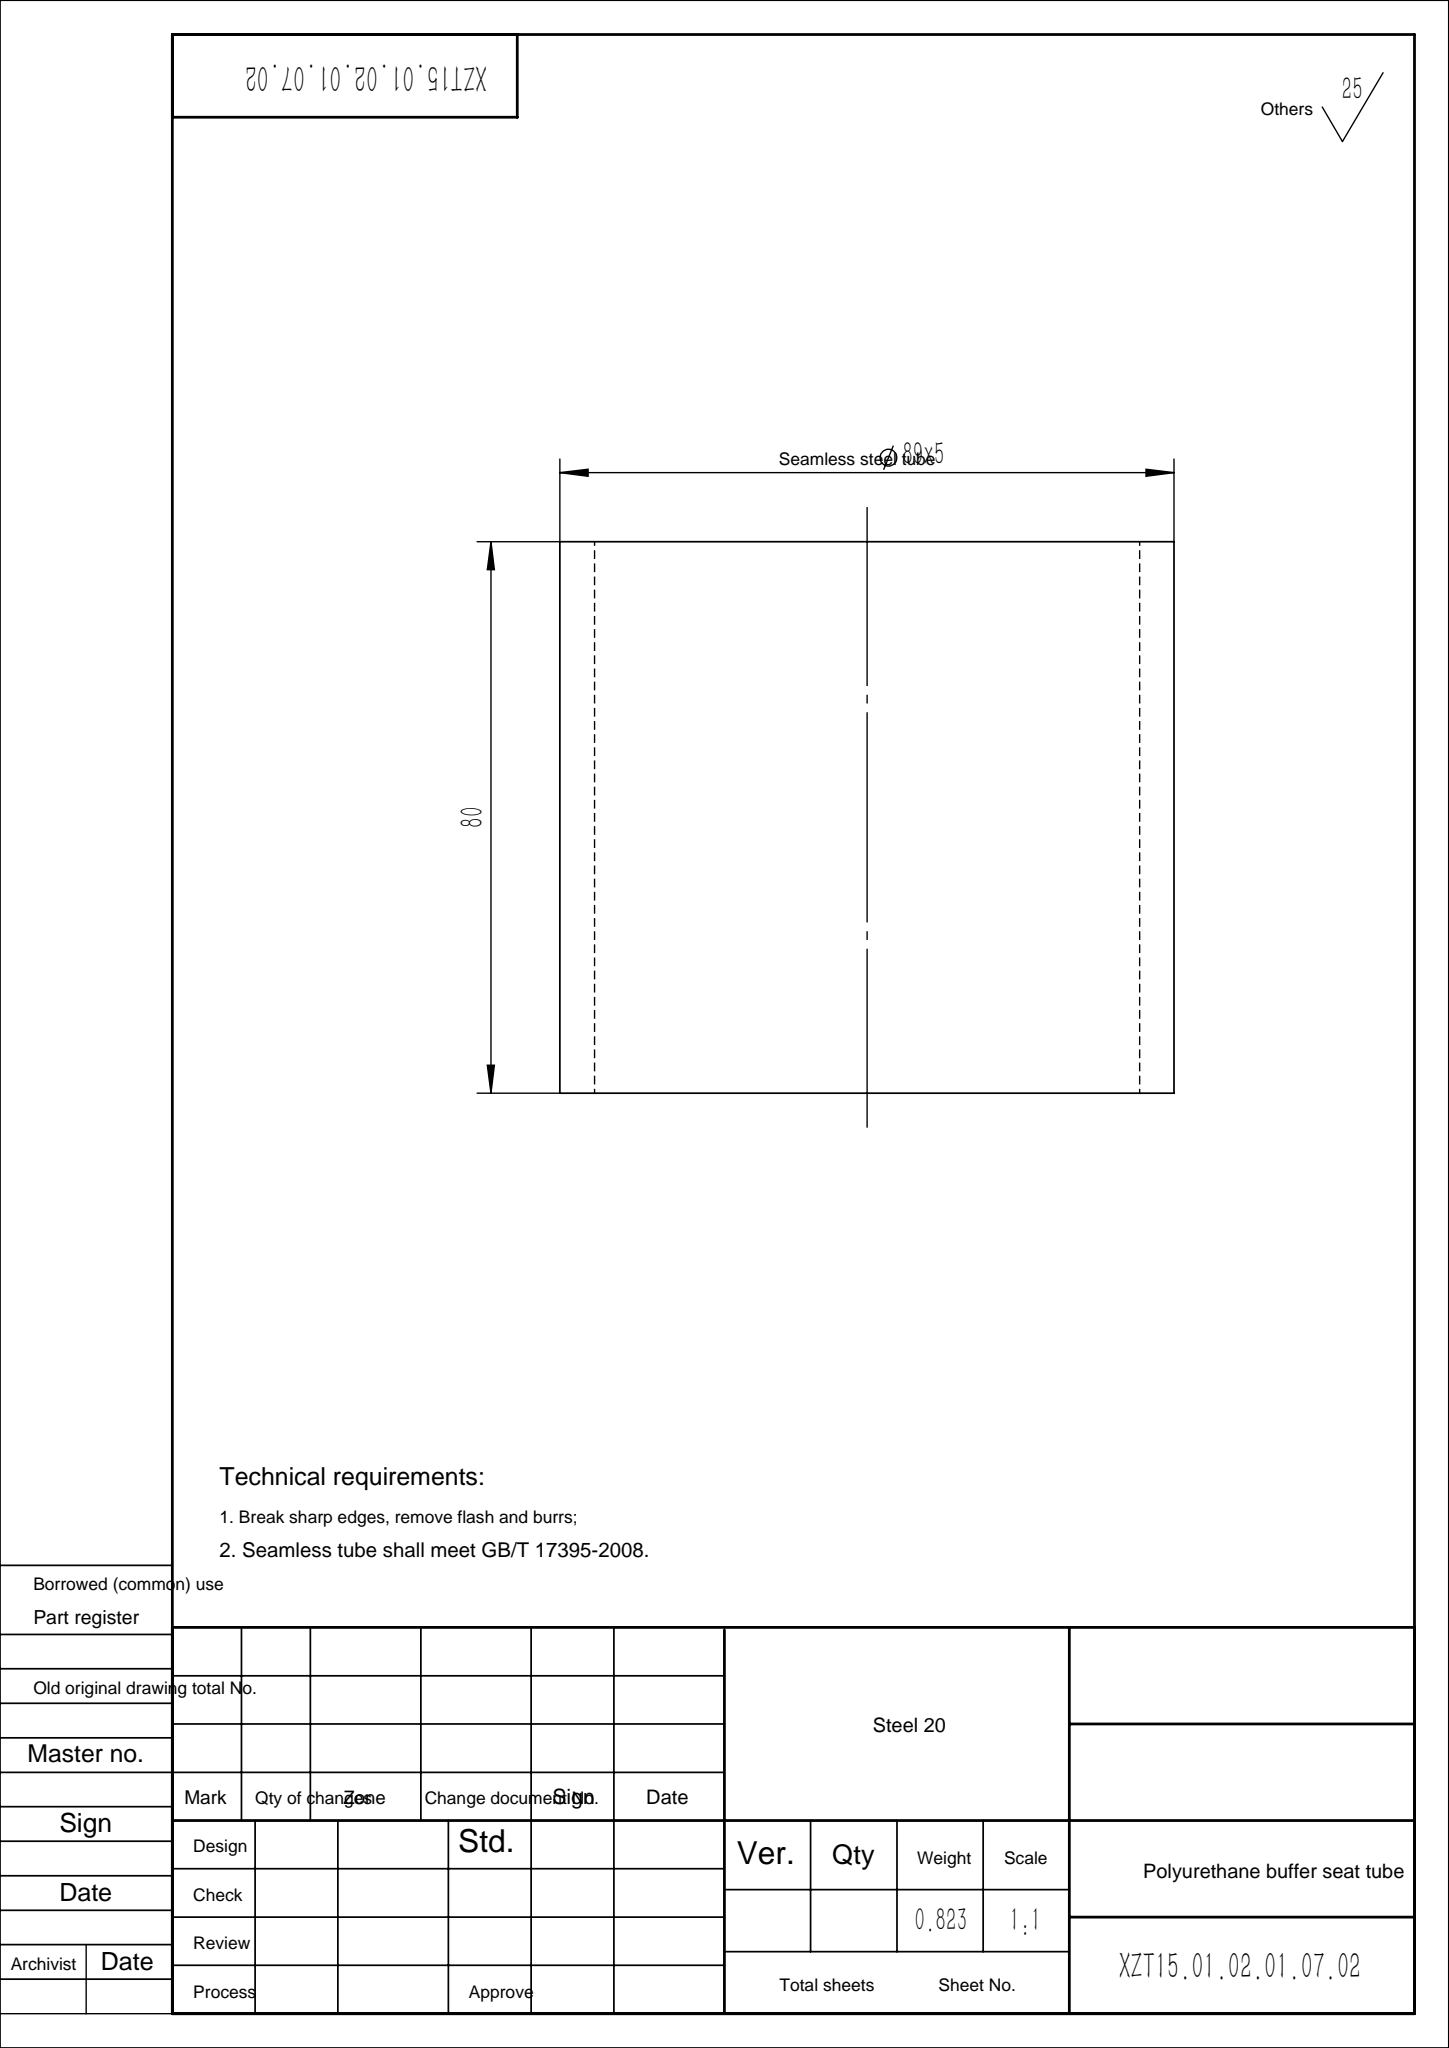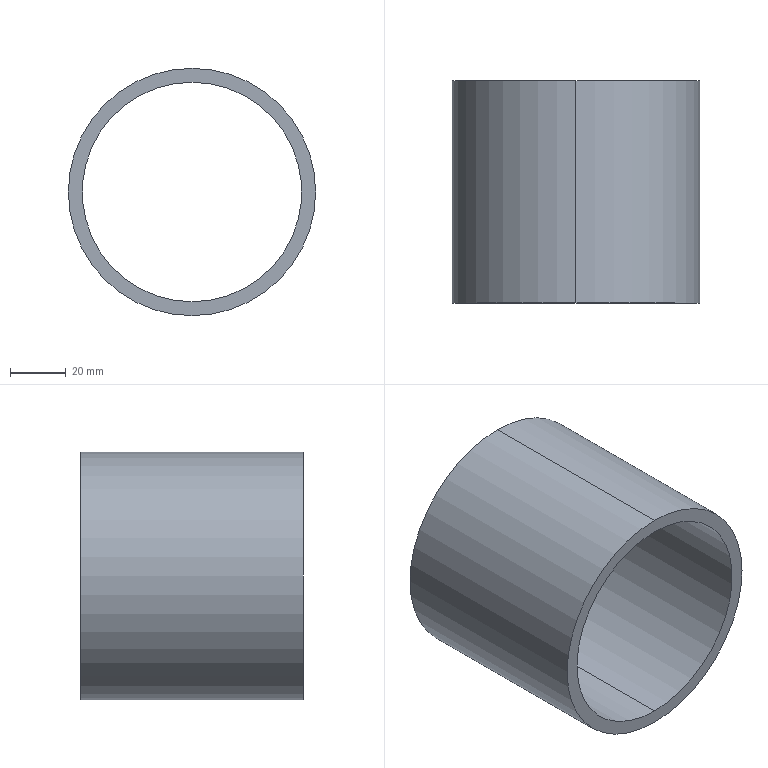Part | SolidWorks | features Extrusion 1 | 1 solid | 6 faces | box 89 x 80 x 89 mm | volume 105558 mm3 | cylinder 4 | plane 2 | commonest cylinder face diameters 79 x2 89 x2
STEP:
#1=CARTESIAN_POINT('',(0.,80.,-39.5));
#2=VERTEX_POINT('',#1);
#3=CARTESIAN_POINT('',(0.,80.,39.5));
#4=VERTEX_POINT('',#3);
#5=CARTESIAN_POINT('',(0.,80.,0.));
#6=DIRECTION('',(0.,1.,0.));
#7=DIRECTION('',(0.,0.,1.));
#8=AXIS2_PLACEMENT_3D('',#5,#6,#7);
#9=CIRCLE('',#8,39.5);
#10=EDGE_CURVE('',#2,#4,#9,.T.);
#11=ORIENTED_EDGE('',*,*,#10,.T.);
#12=CARTESIAN_POINT('',(0.,0.,39.5));
#13=VERTEX_POINT('',#12);
#14=CARTESIAN_POINT('',(0.,80.,39.5));
#15=DIRECTION('',(0.,-1.,0.));
#16=VECTOR('',#15,1000.);
#17=LINE('',#14,#16);
#18=EDGE_CURVE('',#4,#13,#17,.T.);
#19=ORIENTED_EDGE('',*,*,#18,.T.);
#20=CARTESIAN_POINT('',(0.,0.,-39.5));
#21=VERTEX_POINT('',#20);
#22=CARTESIAN_POINT('',(0.,0.,0.));
#23=DIRECTION('',(0.,1.,0.));
#24=DIRECTION('',(0.,0.,1.));
#25=AXIS2_PLACEMENT_3D('',#22,#23,#24);
#26=CIRCLE('',#25,39.5);
#27=EDGE_CURVE('',#21,#13,#26,.T.);
#28=ORIENTED_EDGE('',*,*,#27,.F.);
#29=CARTESIAN_POINT('',(0.,80.,-39.5));
#30=DIRECTION('',(0.,-1.,0.));
#31=VECTOR('',#30,1000.);
#32=LINE('',#29,#31);
#33=EDGE_CURVE('',#2,#21,#32,.T.);
#34=ORIENTED_EDGE('',*,*,#33,.F.);
#35=EDGE_LOOP('',(#11,#19,#28,#34));
#36=FACE_OUTER_BOUND('',#35,.T.);
#37=CARTESIAN_POINT('',(0.,80.,0.));
#38=DIRECTION('',(0.,-1.,0.));
#39=DIRECTION('',(0.,0.,-1.));
#40=AXIS2_PLACEMENT_3D('',#37,#38,#39);
#41=CYLINDRICAL_SURFACE('',#40,39.5);
#42=ADVANCED_FACE('',(#36),#41,.F.);
#43=CARTESIAN_POINT('',(0.,80.,44.5));
#44=VERTEX_POINT('',#43);
#45=CARTESIAN_POINT('',(0.,80.,-44.5));
#46=VERTEX_POINT('',#45);
#47=CARTESIAN_POINT('',(0.,80.,0.));
#48=DIRECTION('',(0.,1.,0.));
#49=DIRECTION('',(0.,0.,1.));
#50=AXIS2_PLACEMENT_3D('',#47,#48,#49);
#51=CIRCLE('',#50,44.5);
#52=EDGE_CURVE('',#44,#46,#51,.T.);
#53=ORIENTED_EDGE('',*,*,#52,.F.);
#54=CARTESIAN_POINT('',(0.,0.,44.5));
#55=VERTEX_POINT('',#54);
#56=CARTESIAN_POINT('',(0.,80.,44.5));
#57=DIRECTION('',(0.,-1.,0.));
#58=VECTOR('',#57,1000.);
#59=LINE('',#56,#58);
#60=EDGE_CURVE('',#44,#55,#59,.T.);
#61=ORIENTED_EDGE('',*,*,#60,.T.);
#62=CARTESIAN_POINT('',(0.,0.,-44.5));
#63=VERTEX_POINT('',#62);
#64=CARTESIAN_POINT('',(0.,0.,0.));
#65=DIRECTION('',(0.,1.,0.));
#66=DIRECTION('',(0.,0.,1.));
#67=AXIS2_PLACEMENT_3D('',#64,#65,#66);
#68=CIRCLE('',#67,44.5);
#69=EDGE_CURVE('',#55,#63,#68,.T.);
#70=ORIENTED_EDGE('',*,*,#69,.T.);
#71=CARTESIAN_POINT('',(0.,80.,-44.5));
#72=DIRECTION('',(0.,-1.,0.));
#73=VECTOR('',#72,1000.);
#74=LINE('',#71,#73);
#75=EDGE_CURVE('',#46,#63,#74,.T.);
#76=ORIENTED_EDGE('',*,*,#75,.F.);
#77=EDGE_LOOP('',(#53,#61,#70,#76));
#78=FACE_OUTER_BOUND('',#77,.T.);
#79=CARTESIAN_POINT('',(0.,80.,0.));
#80=DIRECTION('',(0.,-1.,0.));
#81=DIRECTION('',(0.,0.,-1.));
#82=AXIS2_PLACEMENT_3D('',#79,#80,#81);
#83=CYLINDRICAL_SURFACE('',#82,44.5);
#84=ADVANCED_FACE('',(#78),#83,.T.);
#85=CARTESIAN_POINT('',(0.,80.,0.));
#86=DIRECTION('',(0.,1.,0.));
#87=DIRECTION('',(0.,0.,1.));
#88=AXIS2_PLACEMENT_3D('',#85,#86,#87);
#89=CIRCLE('',#88,44.5);
#90=EDGE_CURVE('',#46,#44,#89,.T.);
#91=ORIENTED_EDGE('',*,*,#90,.T.);
#92=ORIENTED_EDGE('',*,*,#52,.T.);
#93=EDGE_LOOP('',(#91,#92));
#94=FACE_OUTER_BOUND('',#93,.T.);
#95=ORIENTED_EDGE('',*,*,#10,.F.);
#96=CARTESIAN_POINT('',(0.,80.,0.));
#97=DIRECTION('',(0.,1.,0.));
#98=DIRECTION('',(0.,0.,1.));
#99=AXIS2_PLACEMENT_3D('',#96,#97,#98);
#100=CIRCLE('',#99,39.5);
#101=EDGE_CURVE('',#4,#2,#100,.T.);
#102=ORIENTED_EDGE('',*,*,#101,.F.);
#103=EDGE_LOOP('',(#95,#102));
#104=FACE_BOUND('',#103,.T.);
#105=CARTESIAN_POINT('',(0.,80.,0.));
#106=DIRECTION('',(0.,1.,0.));
#107=DIRECTION('',(0.,0.,1.));
#108=AXIS2_PLACEMENT_3D('',#105,#106,#107);
#109=PLANE('',#108);
#110=ADVANCED_FACE('',(#94,#104),#109,.T.);
#111=CARTESIAN_POINT('',(0.,0.,0.));
#112=DIRECTION('',(0.,1.,0.));
#113=DIRECTION('',(0.,0.,1.));
#114=AXIS2_PLACEMENT_3D('',#111,#112,#113);
#115=CIRCLE('',#114,44.5);
#116=EDGE_CURVE('',#63,#55,#115,.T.);
#117=ORIENTED_EDGE('',*,*,#116,.F.);
#118=ORIENTED_EDGE('',*,*,#69,.F.);
#119=EDGE_LOOP('',(#117,#118));
#120=FACE_OUTER_BOUND('',#119,.T.);
#121=ORIENTED_EDGE('',*,*,#27,.T.);
#122=CARTESIAN_POINT('',(0.,0.,0.));
#123=DIRECTION('',(0.,1.,0.));
#124=DIRECTION('',(0.,0.,1.));
#125=AXIS2_PLACEMENT_3D('',#122,#123,#124);
#126=CIRCLE('',#125,39.5);
#127=EDGE_CURVE('',#13,#21,#126,.T.);
#128=ORIENTED_EDGE('',*,*,#127,.T.);
#129=EDGE_LOOP('',(#121,#128));
#130=FACE_BOUND('',#129,.T.);
#131=CARTESIAN_POINT('',(0.,0.,0.));
#132=DIRECTION('',(0.,1.,0.));
#133=DIRECTION('',(0.,0.,1.));
#134=AXIS2_PLACEMENT_3D('',#131,#132,#133);
#135=PLANE('',#134);
#136=ADVANCED_FACE('',(#120,#130),#135,.F.);
#137=ORIENTED_EDGE('',*,*,#60,.F.);
#138=ORIENTED_EDGE('',*,*,#90,.F.);
#139=ORIENTED_EDGE('',*,*,#75,.T.);
#140=ORIENTED_EDGE('',*,*,#116,.T.);
#141=EDGE_LOOP('',(#137,#138,#139,#140));
#142=FACE_OUTER_BOUND('',#141,.T.);
#143=CARTESIAN_POINT('',(0.,80.,0.));
#144=DIRECTION('',(0.,-1.,0.));
#145=DIRECTION('',(0.,0.,-1.));
#146=AXIS2_PLACEMENT_3D('',#143,#144,#145);
#147=CYLINDRICAL_SURFACE('',#146,44.5);
#148=ADVANCED_FACE('',(#142),#147,.T.);
#149=ORIENTED_EDGE('',*,*,#18,.F.);
#150=ORIENTED_EDGE('',*,*,#101,.T.);
#151=ORIENTED_EDGE('',*,*,#33,.T.);
#152=ORIENTED_EDGE('',*,*,#127,.F.);
#153=EDGE_LOOP('',(#149,#150,#151,#152));
#154=FACE_OUTER_BOUND('',#153,.T.);
#155=CARTESIAN_POINT('',(0.,80.,0.));
#156=DIRECTION('',(0.,-1.,0.));
#157=DIRECTION('',(0.,0.,-1.));
#158=AXIS2_PLACEMENT_3D('',#155,#156,#157);
#159=CYLINDRICAL_SURFACE('',#158,39.5);
#160=ADVANCED_FACE('',(#154),#159,.F.);
#161=CLOSED_SHELL('',(#42,#84,#110,#136,#148,#160));
#162=MANIFOLD_SOLID_BREP('',#161);
#163=CARTESIAN_POINT('',(0.,0.,0.));
#164=DIRECTION('',(0.,0.,1.));
#165=DIRECTION('',(1.,0.,0.));
#166=AXIS2_PLACEMENT_3D('',#163,#164,#165);
#167=(LENGTH_UNIT()NAMED_UNIT(*)SI_UNIT(.MILLI.,.METRE.));
#168=UNCERTAINTY_MEASURE_WITH_UNIT(LENGTH_MEASURE(0.00001),#167,'','');
#169=(NAMED_UNIT(*)PLANE_ANGLE_UNIT()SI_UNIT($,.RADIAN.));
#170=(NAMED_UNIT(*)SI_UNIT($,.STERADIAN.)SOLID_ANGLE_UNIT());
#171=(GEOMETRIC_REPRESENTATION_CONTEXT(3)GLOBAL_UNCERTAINTY_ASSIGNED_CONTEXT((#168))GLOBAL_UNIT_ASSIGNED_CONTEXT((#167,#169,#170))REPRESENTATION_CONTEXT('',''));
#172=ADVANCED_BREP_SHAPE_REPRESENTATION('',(#162,#166),#171);